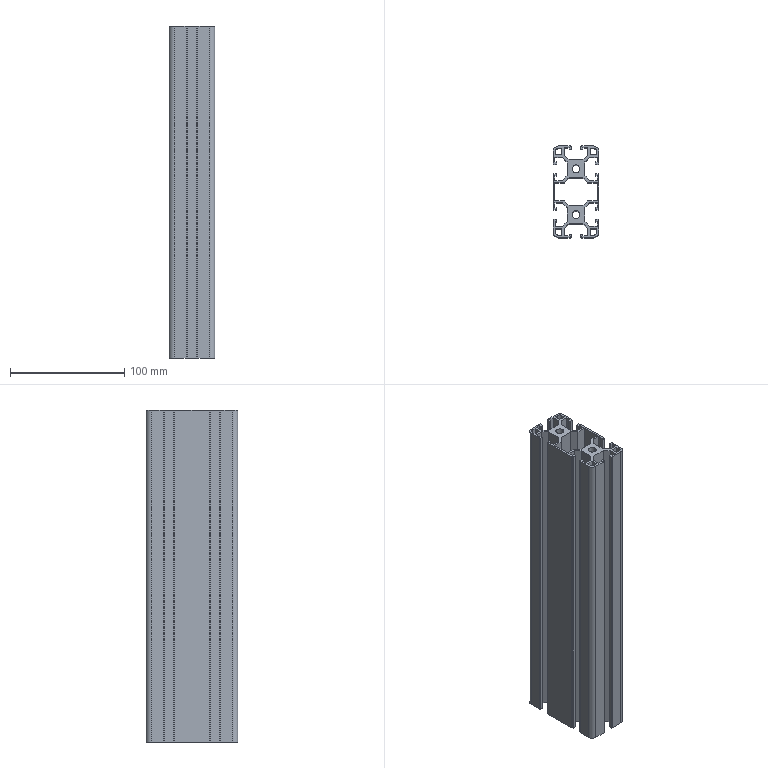Part | SolidWorks | features BaseBody 1 | 1 solid | 155 faces | box 40.002 x 80 x 290 mm | volume 285474 mm3 | plane 142 | cylinder 13 | commonest cylinder face diameters 9 x5 5 x4 6.8 x4